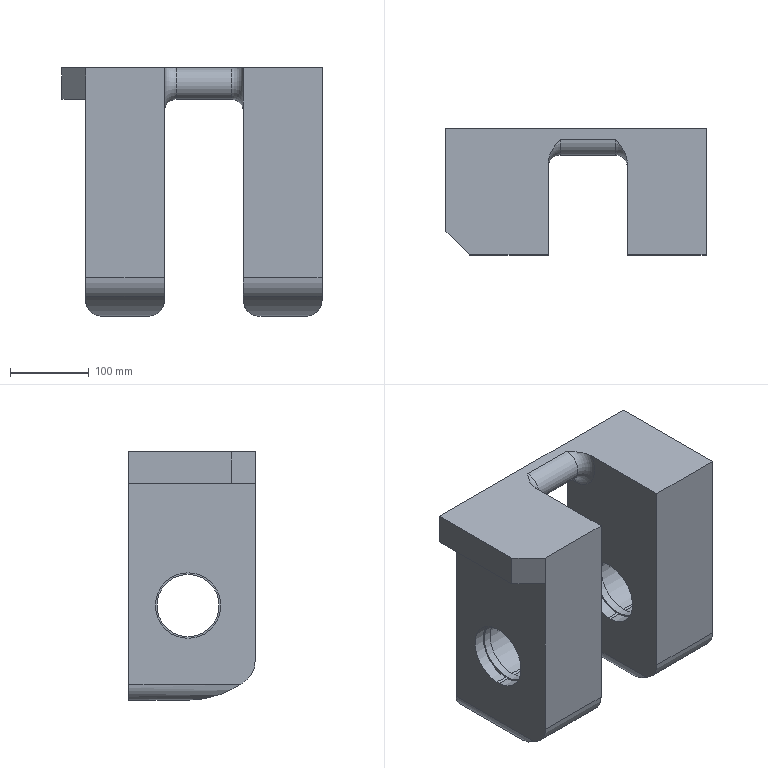Part | NX | features solid 2 | 1 solid | 83 faces | box 330 x 160 x 315 mm | volume 9090029 mm3 | plane 54 | cylinder 27 | torus 2 | commonest cylinder face diameters 83 x12 40 x5 79 x4 30 x2 60 x2 240 x2